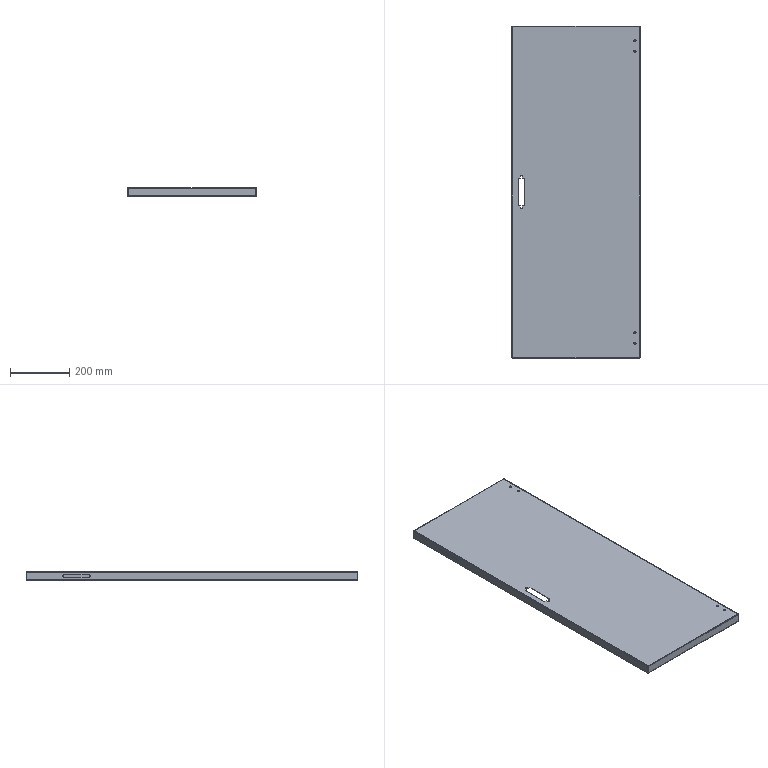Part | 1 solid | 95 faces | box 432 x 1120 x 30 mm | volume 719068 mm3 | plane 50 | cylinder 29 | spline 16 | commonest cylinder face diameters 7 x13 1.473 x8 3.873 x8